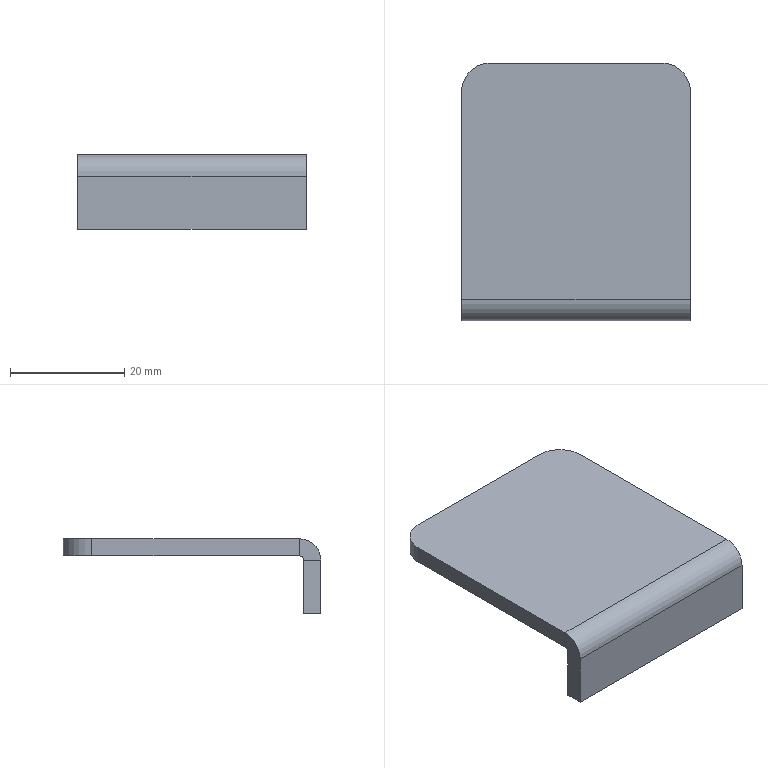Part | SolidWorks | features EdgeFlange 1, Fillet 1, FlatPattern 1, SMBaseFlange 1, SheetMetal 1 | 1 solid | 16 faces | box 40 x 45 x 13 mm | volume 6453 mm3 | plane 12 | cylinder 4 | commonest cylinder face diameters 10 x2 1.473 x1 7.473 x1
STEP:
#1=CARTESIAN_POINT('',(20.,0.,4.263));
#2=VERTEX_POINT('',#1);
#3=CARTESIAN_POINT('',(20.,0.,-5.));
#4=VERTEX_POINT('',#3);
#5=CARTESIAN_POINT('',(20.,0.,5.));
#6=DIRECTION('',(0.,0.,-1.));
#7=VECTOR('',#6,1000.);
#8=LINE('',#5,#7);
#9=EDGE_CURVE('',#2,#4,#8,.T.);
#10=ORIENTED_EDGE('',*,*,#9,.F.);
#11=CARTESIAN_POINT('',(20.,-3.,4.263));
#12=VERTEX_POINT('',#11);
#13=CARTESIAN_POINT('',(20.,0.,4.263));
#14=DIRECTION('',(0.,-1.,0.));
#15=VECTOR('',#14,1000.);
#16=LINE('',#13,#15);
#17=EDGE_CURVE('',#2,#12,#16,.T.);
#18=ORIENTED_EDGE('',*,*,#17,.T.);
#19=CARTESIAN_POINT('',(20.,-3.,-5.));
#20=VERTEX_POINT('',#19);
#21=CARTESIAN_POINT('',(20.,-3.,5.));
#22=DIRECTION('',(0.,0.,-1.));
#23=VECTOR('',#22,1000.);
#24=LINE('',#21,#23);
#25=EDGE_CURVE('',#12,#20,#24,.T.);
#26=ORIENTED_EDGE('',*,*,#25,.T.);
#27=CARTESIAN_POINT('',(20.,-3.,-5.));
#28=DIRECTION('',(0.,1.,0.));
#29=VECTOR('',#28,1000.);
#30=LINE('',#27,#29);
#31=EDGE_CURVE('',#20,#4,#30,.T.);
#32=ORIENTED_EDGE('',*,*,#31,.T.);
#33=EDGE_LOOP('',(#10,#18,#26,#32));
#34=FACE_OUTER_BOUND('',#33,.T.);
#35=CARTESIAN_POINT('',(20.,-3.,5.));
#36=DIRECTION('',(1.,0.,0.));
#37=DIRECTION('',(0.,0.,-1.));
#38=AXIS2_PLACEMENT_3D('',#35,#36,#37);
#39=PLANE('',#38);
#40=ADVANCED_FACE('',(#34),#39,.T.);
#41=ORIENTED_EDGE('',*,*,#25,.F.);
#42=CARTESIAN_POINT('',(-20.,-3.,4.263));
#43=VERTEX_POINT('',#42);
#44=CARTESIAN_POINT('',(20.,-3.,4.263));
#45=DIRECTION('',(-1.,0.,0.));
#46=VECTOR('',#45,1000.);
#47=LINE('',#44,#46);
#48=EDGE_CURVE('',#12,#43,#47,.T.);
#49=ORIENTED_EDGE('',*,*,#48,.T.);
#50=CARTESIAN_POINT('',(-20.,-3.,-5.));
#51=VERTEX_POINT('',#50);
#52=CARTESIAN_POINT('',(-20.,-3.,5.));
#53=DIRECTION('',(0.,0.,1.));
#54=VECTOR('',#53,1000.);
#55=LINE('',#52,#54);
#56=EDGE_CURVE('',#51,#43,#55,.T.);
#57=ORIENTED_EDGE('',*,*,#56,.F.);
#58=CARTESIAN_POINT('',(-20.,-3.,-5.));
#59=DIRECTION('',(-1.,0.,0.));
#60=VECTOR('',#59,1000.);
#61=LINE('',#58,#60);
#62=EDGE_CURVE('',#20,#51,#61,.T.);
#63=ORIENTED_EDGE('',*,*,#62,.F.);
#64=EDGE_LOOP('',(#41,#49,#57,#63));
#65=FACE_OUTER_BOUND('',#64,.T.);
#66=CARTESIAN_POINT('',(0.,-3.,0.));
#67=DIRECTION('',(0.,-1.,0.));
#68=DIRECTION('',(0.,0.,-1.));
#69=AXIS2_PLACEMENT_3D('',#66,#67,#68);
#70=PLANE('',#69);
#71=ADVANCED_FACE('',(#65),#70,.T.);
#72=CARTESIAN_POINT('',(-20.,0.,4.263));
#73=VERTEX_POINT('',#72);
#74=CARTESIAN_POINT('',(20.,0.,4.263));
#75=DIRECTION('',(-1.,0.,0.));
#76=VECTOR('',#75,1000.);
#77=LINE('',#74,#76);
#78=EDGE_CURVE('',#2,#73,#77,.T.);
#79=ORIENTED_EDGE('',*,*,#78,.F.);
#80=ORIENTED_EDGE('',*,*,#9,.T.);
#81=CARTESIAN_POINT('',(-20.,0.,-5.));
#82=VERTEX_POINT('',#81);
#83=CARTESIAN_POINT('',(-20.,0.,-5.));
#84=DIRECTION('',(-1.,0.,0.));
#85=VECTOR('',#84,1000.);
#86=LINE('',#83,#85);
#87=EDGE_CURVE('',#4,#82,#86,.T.);
#88=ORIENTED_EDGE('',*,*,#87,.T.);
#89=CARTESIAN_POINT('',(-20.,0.,5.));
#90=DIRECTION('',(0.,0.,1.));
#91=VECTOR('',#90,1000.);
#92=LINE('',#89,#91);
#93=EDGE_CURVE('',#82,#73,#92,.T.);
#94=ORIENTED_EDGE('',*,*,#93,.T.);
#95=EDGE_LOOP('',(#79,#80,#88,#94));
#96=FACE_OUTER_BOUND('',#95,.T.);
#97=CARTESIAN_POINT('',(0.,0.,0.));
#98=DIRECTION('',(0.,-1.,0.));
#99=DIRECTION('',(0.,0.,-1.));
#100=AXIS2_PLACEMENT_3D('',#97,#98,#99);
#101=PLANE('',#100);
#102=ADVANCED_FACE('',(#96),#101,.F.);
#103=CARTESIAN_POINT('',(-20.,0.,4.263));
#104=DIRECTION('',(0.,-1.,0.));
#105=VECTOR('',#104,1000.);
#106=LINE('',#103,#105);
#107=EDGE_CURVE('',#73,#43,#106,.T.);
#108=ORIENTED_EDGE('',*,*,#107,.F.);
#109=ORIENTED_EDGE('',*,*,#93,.F.);
#110=CARTESIAN_POINT('',(-20.,-3.,-5.));
#111=DIRECTION('',(0.,1.,0.));
#112=VECTOR('',#111,1000.);
#113=LINE('',#110,#112);
#114=EDGE_CURVE('',#51,#82,#113,.T.);
#115=ORIENTED_EDGE('',*,*,#114,.F.);
#116=ORIENTED_EDGE('',*,*,#56,.T.);
#117=EDGE_LOOP('',(#108,#109,#115,#116));
#118=FACE_OUTER_BOUND('',#117,.T.);
#119=CARTESIAN_POINT('',(-20.,-3.,5.));
#120=DIRECTION('',(-1.,0.,0.));
#121=DIRECTION('',(0.,0.,1.));
#122=AXIS2_PLACEMENT_3D('',#119,#120,#121);
#123=PLANE('',#122);
#124=ADVANCED_FACE('',(#118),#123,.T.);
#125=ORIENTED_EDGE('',*,*,#87,.F.);
#126=ORIENTED_EDGE('',*,*,#31,.F.);
#127=ORIENTED_EDGE('',*,*,#62,.T.);
#128=ORIENTED_EDGE('',*,*,#114,.T.);
#129=EDGE_LOOP('',(#125,#126,#127,#128));
#130=FACE_OUTER_BOUND('',#129,.T.);
#131=CARTESIAN_POINT('',(-20.,-3.,-5.));
#132=DIRECTION('',(0.,0.,-1.));
#133=DIRECTION('',(-1.,0.,0.));
#134=AXIS2_PLACEMENT_3D('',#131,#132,#133);
#135=PLANE('',#134);
#136=ADVANCED_FACE('',(#130),#135,.T.);
#137=CARTESIAN_POINT('',(-20.,0.7366,5.));
#138=VERTEX_POINT('',#137);
#139=CARTESIAN_POINT('',(-20.,0.7366,8.));
#140=VERTEX_POINT('',#139);
#141=CARTESIAN_POINT('',(-20.,0.7366,5.));
#142=DIRECTION('',(0.,0.,1.));
#143=VECTOR('',#142,1000.);
#144=LINE('',#141,#143);
#145=EDGE_CURVE('',#138,#140,#144,.T.);
#146=ORIENTED_EDGE('',*,*,#145,.F.);
#147=CARTESIAN_POINT('',(-20.,0.7366,4.263));
#148=DIRECTION('',(-1.,0.,0.));
#149=DIRECTION('',(0.,0.,-1.));
#150=AXIS2_PLACEMENT_3D('',#147,#148,#149);
#151=CIRCLE('',#150,0.7366);
#152=EDGE_CURVE('',#73,#138,#151,.T.);
#153=ORIENTED_EDGE('',*,*,#152,.F.);
#154=ORIENTED_EDGE('',*,*,#107,.T.);
#155=CARTESIAN_POINT('',(-20.,0.7366,4.263));
#156=DIRECTION('',(-1.,0.,0.));
#157=DIRECTION('',(0.,0.,-1.));
#158=AXIS2_PLACEMENT_3D('',#155,#156,#157);
#159=CIRCLE('',#158,3.737);
#160=EDGE_CURVE('',#43,#140,#159,.T.);
#161=ORIENTED_EDGE('',*,*,#160,.T.);
#162=EDGE_LOOP('',(#146,#153,#154,#161));
#163=FACE_OUTER_BOUND('',#162,.T.);
#164=CARTESIAN_POINT('',(-20.,0.7366,4.263));
#165=DIRECTION('',(-1.,0.,0.));
#166=DIRECTION('',(0.,0.,1.));
#167=AXIS2_PLACEMENT_3D('',#164,#165,#166);
#168=PLANE('',#167);
#169=ADVANCED_FACE('',(#163),#168,.T.);
#170=CARTESIAN_POINT('',(20.,0.7366,5.));
#171=VERTEX_POINT('',#170);
#172=CARTESIAN_POINT('',(20.,0.7366,4.263));
#173=DIRECTION('',(1.,0.,0.));
#174=DIRECTION('',(0.,0.,-1.));
#175=AXIS2_PLACEMENT_3D('',#172,#173,#174);
#176=CIRCLE('',#175,0.7366);
#177=EDGE_CURVE('',#171,#2,#176,.T.);
#178=ORIENTED_EDGE('',*,*,#177,.F.);
#179=CARTESIAN_POINT('',(20.,0.7366,8.));
#180=VERTEX_POINT('',#179);
#181=CARTESIAN_POINT('',(20.,0.7366,5.));
#182=DIRECTION('',(0.,0.,1.));
#183=VECTOR('',#182,1000.);
#184=LINE('',#181,#183);
#185=EDGE_CURVE('',#171,#180,#184,.T.);
#186=ORIENTED_EDGE('',*,*,#185,.T.);
#187=CARTESIAN_POINT('',(20.,0.7366,4.263));
#188=DIRECTION('',(1.,0.,0.));
#189=DIRECTION('',(0.,0.,-1.));
#190=AXIS2_PLACEMENT_3D('',#187,#188,#189);
#191=CIRCLE('',#190,3.737);
#192=EDGE_CURVE('',#180,#12,#191,.T.);
#193=ORIENTED_EDGE('',*,*,#192,.T.);
#194=ORIENTED_EDGE('',*,*,#17,.F.);
#195=EDGE_LOOP('',(#178,#186,#193,#194));
#196=FACE_OUTER_BOUND('',#195,.T.);
#197=CARTESIAN_POINT('',(20.,0.7366,4.263));
#198=DIRECTION('',(-1.,0.,0.));
#199=DIRECTION('',(0.,0.,1.));
#200=AXIS2_PLACEMENT_3D('',#197,#198,#199);
#201=PLANE('',#200);
#202=ADVANCED_FACE('',(#196),#201,.F.);
#203=ORIENTED_EDGE('',*,*,#48,.F.);
#204=ORIENTED_EDGE('',*,*,#192,.F.);
#205=CARTESIAN_POINT('',(0.,0.7366,8.));
#206=DIRECTION('',(1.,0.,0.));
#207=VECTOR('',#206,1000.);
#208=LINE('',#205,#207);
#209=EDGE_CURVE('',#140,#180,#208,.T.);
#210=ORIENTED_EDGE('',*,*,#209,.F.);
#211=ORIENTED_EDGE('',*,*,#160,.F.);
#212=EDGE_LOOP('',(#203,#204,#210,#211));
#213=FACE_OUTER_BOUND('',#212,.T.);
#214=CARTESIAN_POINT('',(20.,0.7366,4.263));
#215=DIRECTION('',(1.,0.,0.));
#216=DIRECTION('',(0.,0.,1.));
#217=AXIS2_PLACEMENT_3D('',#214,#215,#216);
#218=CYLINDRICAL_SURFACE('',#217,3.737);
#219=ADVANCED_FACE('',(#213),#218,.T.);
#220=ORIENTED_EDGE('',*,*,#78,.T.);
#221=ORIENTED_EDGE('',*,*,#152,.T.);
#222=CARTESIAN_POINT('',(-20.,0.7366,5.));
#223=DIRECTION('',(1.,0.,0.));
#224=VECTOR('',#223,1000.);
#225=LINE('',#222,#224);
#226=EDGE_CURVE('',#138,#171,#225,.T.);
#227=ORIENTED_EDGE('',*,*,#226,.T.);
#228=ORIENTED_EDGE('',*,*,#177,.T.);
#229=EDGE_LOOP('',(#220,#221,#227,#228));
#230=FACE_OUTER_BOUND('',#229,.T.);
#231=CARTESIAN_POINT('',(20.,0.7366,4.263));
#232=DIRECTION('',(1.,0.,0.));
#233=DIRECTION('',(0.,0.,1.));
#234=AXIS2_PLACEMENT_3D('',#231,#232,#233);
#235=CYLINDRICAL_SURFACE('',#234,0.7366);
#236=ADVANCED_FACE('',(#230),#235,.F.);
#237=CARTESIAN_POINT('',(20.,37.,5.));
#238=VERTEX_POINT('',#237);
#239=CARTESIAN_POINT('',(20.,0.,5.));
#240=DIRECTION('',(0.,-1.,0.));
#241=VECTOR('',#240,1000.);
#242=LINE('',#239,#241);
#243=EDGE_CURVE('',#238,#171,#242,.T.);
#244=ORIENTED_EDGE('',*,*,#243,.F.);
#245=CARTESIAN_POINT('',(20.,37.,8.));
#246=VERTEX_POINT('',#245);
#247=CARTESIAN_POINT('',(20.,37.,8.));
#248=DIRECTION('',(0.,0.,1.));
#249=VECTOR('',#248,1000.);
#250=LINE('',#247,#249);
#251=EDGE_CURVE('',#238,#246,#250,.T.);
#252=ORIENTED_EDGE('',*,*,#251,.T.);
#253=CARTESIAN_POINT('',(20.,0.,8.));
#254=DIRECTION('',(0.,-1.,0.));
#255=VECTOR('',#254,1000.);
#256=LINE('',#253,#255);
#257=EDGE_CURVE('',#246,#180,#256,.T.);
#258=ORIENTED_EDGE('',*,*,#257,.T.);
#259=ORIENTED_EDGE('',*,*,#185,.F.);
#260=EDGE_LOOP('',(#244,#252,#258,#259));
#261=FACE_OUTER_BOUND('',#260,.T.);
#262=CARTESIAN_POINT('',(20.,0.,8.));
#263=DIRECTION('',(1.,0.,0.));
#264=DIRECTION('',(0.,0.,-1.));
#265=AXIS2_PLACEMENT_3D('',#262,#263,#264);
#266=PLANE('',#265);
#267=ADVANCED_FACE('',(#261),#266,.T.);
#268=CARTESIAN_POINT('',(-20.,37.,8.));
#269=VERTEX_POINT('',#268);
#270=CARTESIAN_POINT('',(-20.,42.,8.));
#271=DIRECTION('',(0.,1.,0.));
#272=VECTOR('',#271,1000.);
#273=LINE('',#270,#272);
#274=EDGE_CURVE('',#140,#269,#273,.T.);
#275=ORIENTED_EDGE('',*,*,#274,.T.);
#276=CARTESIAN_POINT('',(-20.,37.,5.));
#277=VERTEX_POINT('',#276);
#278=CARTESIAN_POINT('',(-20.,37.,8.));
#279=DIRECTION('',(0.,0.,-1.));
#280=VECTOR('',#279,1000.);
#281=LINE('',#278,#280);
#282=EDGE_CURVE('',#269,#277,#281,.T.);
#283=ORIENTED_EDGE('',*,*,#282,.T.);
#284=CARTESIAN_POINT('',(-20.,42.,5.));
#285=DIRECTION('',(0.,1.,0.));
#286=VECTOR('',#285,1000.);
#287=LINE('',#284,#286);
#288=EDGE_CURVE('',#138,#277,#287,.T.);
#289=ORIENTED_EDGE('',*,*,#288,.F.);
#290=ORIENTED_EDGE('',*,*,#145,.T.);
#291=EDGE_LOOP('',(#275,#283,#289,#290));
#292=FACE_OUTER_BOUND('',#291,.T.);
#293=CARTESIAN_POINT('',(-20.,42.,8.));
#294=DIRECTION('',(-1.,0.,0.));
#295=DIRECTION('',(0.,0.,1.));
#296=AXIS2_PLACEMENT_3D('',#293,#294,#295);
#297=PLANE('',#296);
#298=ADVANCED_FACE('',(#292),#297,.T.);
#299=ORIENTED_EDGE('',*,*,#257,.F.);
#300=CARTESIAN_POINT('',(15.,42.,8.));
#301=VERTEX_POINT('',#300);
#302=CARTESIAN_POINT('',(15.,37.,8.));
#303=DIRECTION('',(0.,0.,1.));
#304=DIRECTION('',(0.,-1.,0.));
#305=AXIS2_PLACEMENT_3D('',#302,#303,#304);
#306=CIRCLE('',#305,5.);
#307=EDGE_CURVE('',#246,#301,#306,.T.);
#308=ORIENTED_EDGE('',*,*,#307,.T.);
#309=CARTESIAN_POINT('',(-15.,42.,8.));
#310=VERTEX_POINT('',#309);
#311=CARTESIAN_POINT('',(20.,42.,8.));
#312=DIRECTION('',(1.,0.,0.));
#313=VECTOR('',#312,1000.);
#314=LINE('',#311,#313);
#315=EDGE_CURVE('',#310,#301,#314,.T.);
#316=ORIENTED_EDGE('',*,*,#315,.F.);
#317=CARTESIAN_POINT('',(-15.,37.,8.));
#318=DIRECTION('',(0.,0.,1.));
#319=DIRECTION('',(0.,-1.,0.));
#320=AXIS2_PLACEMENT_3D('',#317,#318,#319);
#321=CIRCLE('',#320,5.);
#322=EDGE_CURVE('',#310,#269,#321,.T.);
#323=ORIENTED_EDGE('',*,*,#322,.T.);
#324=ORIENTED_EDGE('',*,*,#274,.F.);
#325=ORIENTED_EDGE('',*,*,#209,.T.);
#326=EDGE_LOOP('',(#299,#308,#316,#323,#324,#325));
#327=FACE_OUTER_BOUND('',#326,.T.);
#328=CARTESIAN_POINT('',(0.,0.,8.));
#329=DIRECTION('',(0.,0.,1.));
#330=DIRECTION('',(0.,-1.,0.));
#331=AXIS2_PLACEMENT_3D('',#328,#329,#330);
#332=PLANE('',#331);
#333=ADVANCED_FACE('',(#327),#332,.T.);
#334=CARTESIAN_POINT('',(-15.,42.,5.));
#335=VERTEX_POINT('',#334);
#336=CARTESIAN_POINT('',(15.,42.,5.));
#337=VERTEX_POINT('',#336);
#338=CARTESIAN_POINT('',(20.,42.,5.));
#339=DIRECTION('',(1.,0.,0.));
#340=VECTOR('',#339,1000.);
#341=LINE('',#338,#340);
#342=EDGE_CURVE('',#335,#337,#341,.T.);
#343=ORIENTED_EDGE('',*,*,#342,.T.);
#344=CARTESIAN_POINT('',(15.,37.,5.));
#345=DIRECTION('',(0.,0.,-1.));
#346=DIRECTION('',(0.,-1.,0.));
#347=AXIS2_PLACEMENT_3D('',#344,#345,#346);
#348=CIRCLE('',#347,5.);
#349=EDGE_CURVE('',#337,#238,#348,.T.);
#350=ORIENTED_EDGE('',*,*,#349,.T.);
#351=ORIENTED_EDGE('',*,*,#243,.T.);
#352=ORIENTED_EDGE('',*,*,#226,.F.);
#353=ORIENTED_EDGE('',*,*,#288,.T.);
#354=CARTESIAN_POINT('',(-15.,37.,5.));
#355=DIRECTION('',(0.,0.,-1.));
#356=DIRECTION('',(0.,-1.,0.));
#357=AXIS2_PLACEMENT_3D('',#354,#355,#356);
#358=CIRCLE('',#357,5.);
#359=EDGE_CURVE('',#277,#335,#358,.T.);
#360=ORIENTED_EDGE('',*,*,#359,.T.);
#361=EDGE_LOOP('',(#343,#350,#351,#352,#353,#360));
#362=FACE_OUTER_BOUND('',#361,.T.);
#363=CARTESIAN_POINT('',(0.,0.,5.));
#364=DIRECTION('',(0.,0.,1.));
#365=DIRECTION('',(0.,-1.,0.));
#366=AXIS2_PLACEMENT_3D('',#363,#364,#365);
#367=PLANE('',#366);
#368=ADVANCED_FACE('',(#362),#367,.F.);
#369=ORIENTED_EDGE('',*,*,#315,.T.);
#370=CARTESIAN_POINT('',(15.,42.,8.));
#371=DIRECTION('',(0.,0.,-1.));
#372=VECTOR('',#371,1000.);
#373=LINE('',#370,#372);
#374=EDGE_CURVE('',#301,#337,#373,.T.);
#375=ORIENTED_EDGE('',*,*,#374,.T.);
#376=ORIENTED_EDGE('',*,*,#342,.F.);
#377=CARTESIAN_POINT('',(-15.,42.,8.));
#378=DIRECTION('',(0.,0.,1.));
#379=VECTOR('',#378,1000.);
#380=LINE('',#377,#379);
#381=EDGE_CURVE('',#335,#310,#380,.T.);
#382=ORIENTED_EDGE('',*,*,#381,.T.);
#383=EDGE_LOOP('',(#369,#375,#376,#382));
#384=FACE_OUTER_BOUND('',#383,.T.);
#385=CARTESIAN_POINT('',(20.,42.,8.));
#386=DIRECTION('',(0.,1.,0.));
#387=DIRECTION('',(0.,0.,1.));
#388=AXIS2_PLACEMENT_3D('',#385,#386,#387);
#389=PLANE('',#388);
#390=ADVANCED_FACE('',(#384),#389,.T.);
#391=ORIENTED_EDGE('',*,*,#307,.F.);
#392=ORIENTED_EDGE('',*,*,#251,.F.);
#393=ORIENTED_EDGE('',*,*,#349,.F.);
#394=ORIENTED_EDGE('',*,*,#374,.F.);
#395=EDGE_LOOP('',(#391,#392,#393,#394));
#396=FACE_OUTER_BOUND('',#395,.T.);
#397=CARTESIAN_POINT('',(15.,37.,8.));
#398=DIRECTION('',(0.,0.,-1.));
#399=DIRECTION('',(0.,1.,0.));
#400=AXIS2_PLACEMENT_3D('',#397,#398,#399);
#401=CYLINDRICAL_SURFACE('',#400,5.);
#402=ADVANCED_FACE('',(#396),#401,.T.);
#403=ORIENTED_EDGE('',*,*,#322,.F.);
#404=ORIENTED_EDGE('',*,*,#381,.F.);
#405=ORIENTED_EDGE('',*,*,#359,.F.);
#406=ORIENTED_EDGE('',*,*,#282,.F.);
#407=EDGE_LOOP('',(#403,#404,#405,#406));
#408=FACE_OUTER_BOUND('',#407,.T.);
#409=CARTESIAN_POINT('',(-15.,37.,8.));
#410=DIRECTION('',(0.,0.,-1.));
#411=DIRECTION('',(0.,1.,0.));
#412=AXIS2_PLACEMENT_3D('',#409,#410,#411);
#413=CYLINDRICAL_SURFACE('',#412,5.);
#414=ADVANCED_FACE('',(#408),#413,.T.);
#415=CLOSED_SHELL('',(#40,#71,#102,#124,#136,#169,#202,#219,#236,#267,#298,#333,#368,#390,#402,#414));
#416=MANIFOLD_SOLID_BREP('',#415);
#417=CARTESIAN_POINT('',(0.,0.,0.));
#418=DIRECTION('',(0.,0.,1.));
#419=DIRECTION('',(1.,0.,0.));
#420=AXIS2_PLACEMENT_3D('',#417,#418,#419);
#421=(LENGTH_UNIT()NAMED_UNIT(*)SI_UNIT(.MILLI.,.METRE.));
#422=UNCERTAINTY_MEASURE_WITH_UNIT(LENGTH_MEASURE(0.00001),#421,'','');
#423=(NAMED_UNIT(*)PLANE_ANGLE_UNIT()SI_UNIT($,.RADIAN.));
#424=(NAMED_UNIT(*)SI_UNIT($,.STERADIAN.)SOLID_ANGLE_UNIT());
#425=(GEOMETRIC_REPRESENTATION_CONTEXT(3)GLOBAL_UNCERTAINTY_ASSIGNED_CONTEXT((#422))GLOBAL_UNIT_ASSIGNED_CONTEXT((#421,#423,#424))REPRESENTATION_CONTEXT('',''));
#426=ADVANCED_BREP_SHAPE_REPRESENTATION('',(#416,#420),#425);